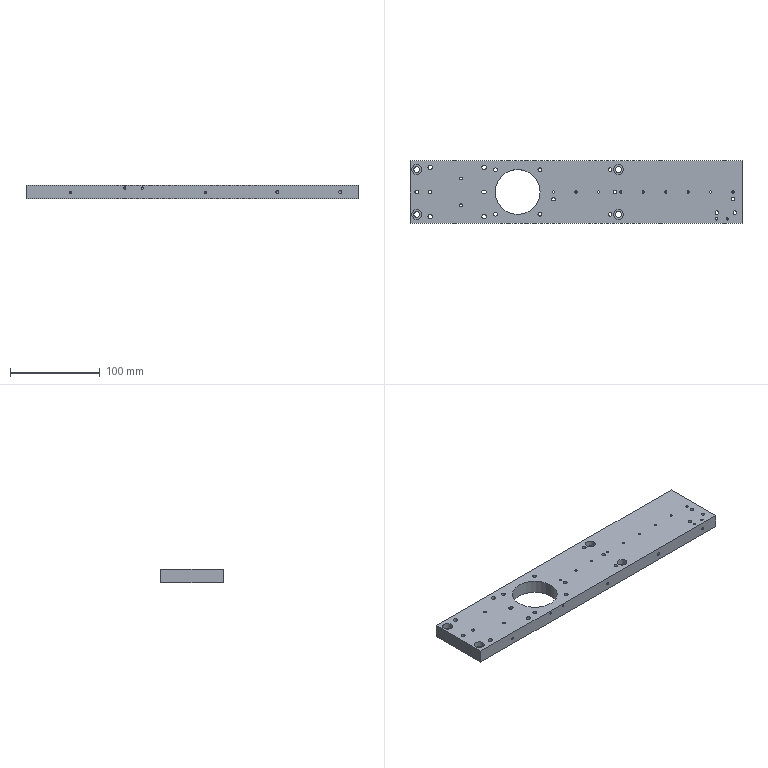Part | 1 solid | 77 faces | box 370 x 70 x 15 mm | volume 349756 mm3 | cylinder 53 | plane 12 | cone 12 | commonest cylinder face diameters 2.5 x19 4 x11 3.3 x6 4.2 x4 5 x4 6.6 x4